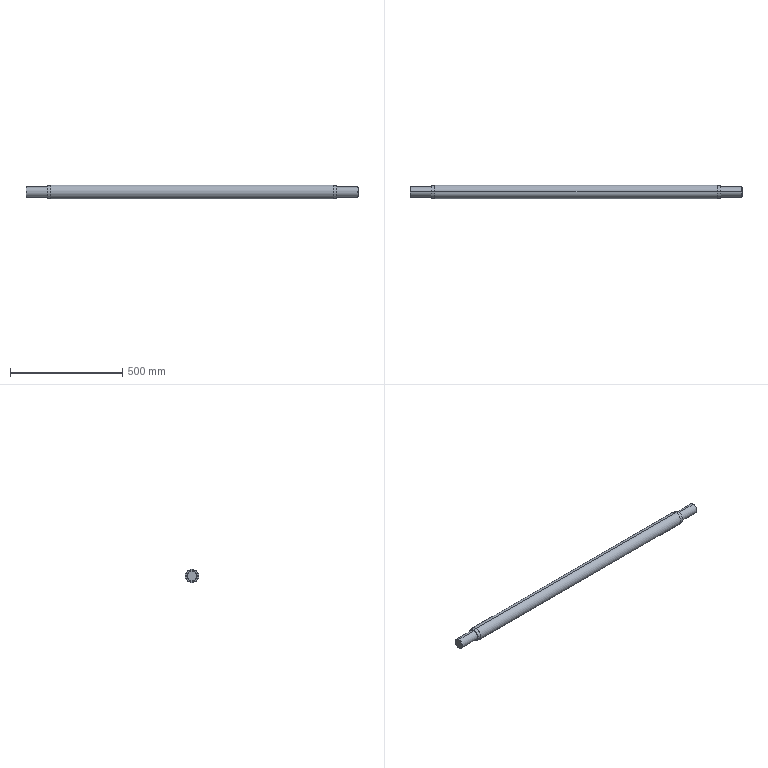Part | SolidWorks | features BaseBody 1 | 1 solid | 20 faces | box 1480 x 60 x 60 mm | volume 3935884 mm3 | cylinder 10 | plane 6 | cone 4 | commonest cylinder face diameters 45 x4 55 x4 60 x2
STEP:
#1=CARTESIAN_POINT('',(1595.073,277.036,21.5));
#2=VERTEX_POINT('',#1);
#3=CARTESIAN_POINT('',(1595.073,277.036,-21.5));
#4=VERTEX_POINT('',#3);
#5=CARTESIAN_POINT('',(1595.073,277.036,0.));
#6=DIRECTION('',(-1.,0.,0.));
#7=DIRECTION('',(0.,0.,1.));
#8=AXIS2_PLACEMENT_3D('',#5,#6,#7);
#9=CIRCLE('',#8,21.5);
#10=EDGE_CURVE('',#2,#4,#9,.T.);
#11=ORIENTED_EDGE('',*,*,#10,.T.);
#12=CARTESIAN_POINT('',(1594.073,277.036,-22.5));
#13=VERTEX_POINT('',#12);
#14=CARTESIAN_POINT('',(1595.073,277.036,-21.5));
#15=DIRECTION('',(-0.7071,0.,-0.7071));
#16=VECTOR('',#15,1000.);
#17=LINE('',#14,#16);
#18=EDGE_CURVE('',#4,#13,#17,.T.);
#19=ORIENTED_EDGE('',*,*,#18,.T.);
#20=CARTESIAN_POINT('',(1594.073,277.036,22.5));
#21=VERTEX_POINT('',#20);
#22=CARTESIAN_POINT('',(1594.073,277.036,0.));
#23=DIRECTION('',(-1.,0.,0.));
#24=DIRECTION('',(0.,0.,1.));
#25=AXIS2_PLACEMENT_3D('',#22,#23,#24);
#26=CIRCLE('',#25,22.5);
#27=EDGE_CURVE('',#21,#13,#26,.T.);
#28=ORIENTED_EDGE('',*,*,#27,.F.);
#29=CARTESIAN_POINT('',(1595.073,277.036,21.5));
#30=DIRECTION('',(-0.7071,0.,0.7071));
#31=VECTOR('',#30,1000.);
#32=LINE('',#29,#31);
#33=EDGE_CURVE('',#2,#21,#32,.T.);
#34=ORIENTED_EDGE('',*,*,#33,.F.);
#35=EDGE_LOOP('',(#11,#19,#28,#34));
#36=FACE_OUTER_BOUND('',#35,.T.);
#37=CARTESIAN_POINT('',(1595.073,277.036,0.));
#38=DIRECTION('',(-1.,0.,0.));
#39=DIRECTION('',(0.,0.,1.));
#40=AXIS2_PLACEMENT_3D('',#37,#38,#39);
#41=CONICAL_SURFACE('',#40,21.5,0.7854);
#42=ADVANCED_FACE('',(#36),#41,.T.);
#43=ORIENTED_EDGE('',*,*,#27,.T.);
#44=CARTESIAN_POINT('',(1500.073,277.036,-22.5));
#45=VERTEX_POINT('',#44);
#46=CARTESIAN_POINT('',(221.073,277.036,-22.5));
#47=DIRECTION('',(-1.,0.,0.));
#48=VECTOR('',#47,1000.);
#49=LINE('',#46,#48);
#50=EDGE_CURVE('',#13,#45,#49,.T.);
#51=ORIENTED_EDGE('',*,*,#50,.T.);
#52=CARTESIAN_POINT('',(1500.073,277.036,22.5));
#53=VERTEX_POINT('',#52);
#54=CARTESIAN_POINT('',(1500.073,277.036,0.));
#55=DIRECTION('',(-1.,0.,0.));
#56=DIRECTION('',(0.,0.,1.));
#57=AXIS2_PLACEMENT_3D('',#54,#55,#56);
#58=CIRCLE('',#57,22.5);
#59=EDGE_CURVE('',#53,#45,#58,.T.);
#60=ORIENTED_EDGE('',*,*,#59,.F.);
#61=CARTESIAN_POINT('',(221.073,277.036,22.5));
#62=DIRECTION('',(-1.,0.,0.));
#63=VECTOR('',#62,1000.);
#64=LINE('',#61,#63);
#65=EDGE_CURVE('',#21,#53,#64,.T.);
#66=ORIENTED_EDGE('',*,*,#65,.F.);
#67=EDGE_LOOP('',(#43,#51,#60,#66));
#68=FACE_OUTER_BOUND('',#67,.T.);
#69=CARTESIAN_POINT('',(221.073,277.036,0.));
#70=DIRECTION('',(-1.,0.,0.));
#71=DIRECTION('',(0.,0.,1.));
#72=AXIS2_PLACEMENT_3D('',#69,#70,#71);
#73=CYLINDRICAL_SURFACE('',#72,22.5);
#74=ADVANCED_FACE('',(#68),#73,.T.);
#75=CARTESIAN_POINT('',(1500.073,277.036,27.5));
#76=VERTEX_POINT('',#75);
#77=CARTESIAN_POINT('',(1500.073,277.036,-27.5));
#78=VERTEX_POINT('',#77);
#79=CARTESIAN_POINT('',(1500.073,277.036,0.));
#80=DIRECTION('',(-1.,0.,0.));
#81=DIRECTION('',(0.,0.,1.));
#82=AXIS2_PLACEMENT_3D('',#79,#80,#81);
#83=CIRCLE('',#82,27.5);
#84=EDGE_CURVE('',#76,#78,#83,.T.);
#85=ORIENTED_EDGE('',*,*,#84,.T.);
#86=CARTESIAN_POINT('',(1485.073,277.036,-27.5));
#87=VERTEX_POINT('',#86);
#88=CARTESIAN_POINT('',(221.073,277.036,-27.5));
#89=DIRECTION('',(-1.,0.,0.));
#90=VECTOR('',#89,1000.);
#91=LINE('',#88,#90);
#92=EDGE_CURVE('',#78,#87,#91,.T.);
#93=ORIENTED_EDGE('',*,*,#92,.T.);
#94=CARTESIAN_POINT('',(1485.073,277.036,27.5));
#95=VERTEX_POINT('',#94);
#96=CARTESIAN_POINT('',(1485.073,277.036,0.));
#97=DIRECTION('',(-1.,0.,0.));
#98=DIRECTION('',(0.,0.,1.));
#99=AXIS2_PLACEMENT_3D('',#96,#97,#98);
#100=CIRCLE('',#99,27.5);
#101=EDGE_CURVE('',#95,#87,#100,.T.);
#102=ORIENTED_EDGE('',*,*,#101,.F.);
#103=CARTESIAN_POINT('',(221.073,277.036,27.5));
#104=DIRECTION('',(-1.,0.,0.));
#105=VECTOR('',#104,1000.);
#106=LINE('',#103,#105);
#107=EDGE_CURVE('',#76,#95,#106,.T.);
#108=ORIENTED_EDGE('',*,*,#107,.F.);
#109=EDGE_LOOP('',(#85,#93,#102,#108));
#110=FACE_OUTER_BOUND('',#109,.T.);
#111=CARTESIAN_POINT('',(221.073,277.036,0.));
#112=DIRECTION('',(-1.,0.,0.));
#113=DIRECTION('',(0.,0.,1.));
#114=AXIS2_PLACEMENT_3D('',#111,#112,#113);
#115=CYLINDRICAL_SURFACE('',#114,27.5);
#116=ADVANCED_FACE('',(#110),#115,.T.);
#117=CARTESIAN_POINT('',(1485.073,277.036,30.));
#118=VERTEX_POINT('',#117);
#119=CARTESIAN_POINT('',(1485.073,277.036,-30.));
#120=VERTEX_POINT('',#119);
#121=CARTESIAN_POINT('',(1485.073,277.036,0.));
#122=DIRECTION('',(-1.,0.,0.));
#123=DIRECTION('',(0.,0.,1.));
#124=AXIS2_PLACEMENT_3D('',#121,#122,#123);
#125=CIRCLE('',#124,30.);
#126=EDGE_CURVE('',#118,#120,#125,.T.);
#127=ORIENTED_EDGE('',*,*,#126,.T.);
#128=CARTESIAN_POINT('',(225.073,277.036,-30.));
#129=VERTEX_POINT('',#128);
#130=CARTESIAN_POINT('',(221.073,277.036,-30.));
#131=DIRECTION('',(-1.,0.,0.));
#132=VECTOR('',#131,1000.);
#133=LINE('',#130,#132);
#134=EDGE_CURVE('',#120,#129,#133,.T.);
#135=ORIENTED_EDGE('',*,*,#134,.T.);
#136=CARTESIAN_POINT('',(225.073,277.036,30.));
#137=VERTEX_POINT('',#136);
#138=CARTESIAN_POINT('',(225.073,277.036,0.));
#139=DIRECTION('',(-1.,0.,0.));
#140=DIRECTION('',(0.,0.,1.));
#141=AXIS2_PLACEMENT_3D('',#138,#139,#140);
#142=CIRCLE('',#141,30.);
#143=EDGE_CURVE('',#137,#129,#142,.T.);
#144=ORIENTED_EDGE('',*,*,#143,.F.);
#145=CARTESIAN_POINT('',(221.073,277.036,30.));
#146=DIRECTION('',(-1.,0.,0.));
#147=VECTOR('',#146,1000.);
#148=LINE('',#145,#147);
#149=EDGE_CURVE('',#118,#137,#148,.T.);
#150=ORIENTED_EDGE('',*,*,#149,.F.);
#151=EDGE_LOOP('',(#127,#135,#144,#150));
#152=FACE_OUTER_BOUND('',#151,.T.);
#153=CARTESIAN_POINT('',(221.073,277.036,0.));
#154=DIRECTION('',(-1.,0.,0.));
#155=DIRECTION('',(0.,0.,1.));
#156=AXIS2_PLACEMENT_3D('',#153,#154,#155);
#157=CYLINDRICAL_SURFACE('',#156,30.);
#158=ADVANCED_FACE('',(#152),#157,.T.);
#159=CARTESIAN_POINT('',(225.073,277.036,27.5));
#160=VERTEX_POINT('',#159);
#161=CARTESIAN_POINT('',(225.073,277.036,-27.5));
#162=VERTEX_POINT('',#161);
#163=CARTESIAN_POINT('',(225.073,277.036,0.));
#164=DIRECTION('',(-1.,0.,0.));
#165=DIRECTION('',(0.,0.,1.));
#166=AXIS2_PLACEMENT_3D('',#163,#164,#165);
#167=CIRCLE('',#166,27.5);
#168=EDGE_CURVE('',#160,#162,#167,.T.);
#169=ORIENTED_EDGE('',*,*,#168,.T.);
#170=CARTESIAN_POINT('',(210.073,277.036,-27.5));
#171=VERTEX_POINT('',#170);
#172=CARTESIAN_POINT('',(221.073,277.036,-27.5));
#173=DIRECTION('',(-1.,0.,0.));
#174=VECTOR('',#173,1000.);
#175=LINE('',#172,#174);
#176=EDGE_CURVE('',#162,#171,#175,.T.);
#177=ORIENTED_EDGE('',*,*,#176,.T.);
#178=CARTESIAN_POINT('',(210.073,277.036,27.5));
#179=VERTEX_POINT('',#178);
#180=CARTESIAN_POINT('',(210.073,277.036,0.));
#181=DIRECTION('',(-1.,0.,0.));
#182=DIRECTION('',(0.,0.,1.));
#183=AXIS2_PLACEMENT_3D('',#180,#181,#182);
#184=CIRCLE('',#183,27.5);
#185=EDGE_CURVE('',#179,#171,#184,.T.);
#186=ORIENTED_EDGE('',*,*,#185,.F.);
#187=CARTESIAN_POINT('',(221.073,277.036,27.5));
#188=DIRECTION('',(-1.,0.,0.));
#189=VECTOR('',#188,1000.);
#190=LINE('',#187,#189);
#191=EDGE_CURVE('',#160,#179,#190,.T.);
#192=ORIENTED_EDGE('',*,*,#191,.F.);
#193=EDGE_LOOP('',(#169,#177,#186,#192));
#194=FACE_OUTER_BOUND('',#193,.T.);
#195=CARTESIAN_POINT('',(221.073,277.036,0.));
#196=DIRECTION('',(-1.,0.,0.));
#197=DIRECTION('',(0.,0.,1.));
#198=AXIS2_PLACEMENT_3D('',#195,#196,#197);
#199=CYLINDRICAL_SURFACE('',#198,27.5);
#200=ADVANCED_FACE('',(#194),#199,.T.);
#201=CARTESIAN_POINT('',(210.073,277.036,22.5));
#202=VERTEX_POINT('',#201);
#203=CARTESIAN_POINT('',(210.073,277.036,-22.5));
#204=VERTEX_POINT('',#203);
#205=CARTESIAN_POINT('',(210.073,277.036,0.));
#206=DIRECTION('',(-1.,0.,0.));
#207=DIRECTION('',(0.,0.,1.));
#208=AXIS2_PLACEMENT_3D('',#205,#206,#207);
#209=CIRCLE('',#208,22.5);
#210=EDGE_CURVE('',#202,#204,#209,.T.);
#211=ORIENTED_EDGE('',*,*,#210,.T.);
#212=CARTESIAN_POINT('',(116.073,277.036,-22.5));
#213=VERTEX_POINT('',#212);
#214=CARTESIAN_POINT('',(221.073,277.036,-22.5));
#215=DIRECTION('',(-1.,0.,0.));
#216=VECTOR('',#215,1000.);
#217=LINE('',#214,#216);
#218=EDGE_CURVE('',#204,#213,#217,.T.);
#219=ORIENTED_EDGE('',*,*,#218,.T.);
#220=CARTESIAN_POINT('',(116.073,277.036,22.5));
#221=VERTEX_POINT('',#220);
#222=CARTESIAN_POINT('',(116.073,277.036,0.));
#223=DIRECTION('',(-1.,0.,0.));
#224=DIRECTION('',(0.,0.,1.));
#225=AXIS2_PLACEMENT_3D('',#222,#223,#224);
#226=CIRCLE('',#225,22.5);
#227=EDGE_CURVE('',#221,#213,#226,.T.);
#228=ORIENTED_EDGE('',*,*,#227,.F.);
#229=CARTESIAN_POINT('',(221.073,277.036,22.5));
#230=DIRECTION('',(-1.,0.,0.));
#231=VECTOR('',#230,1000.);
#232=LINE('',#229,#231);
#233=EDGE_CURVE('',#202,#221,#232,.T.);
#234=ORIENTED_EDGE('',*,*,#233,.F.);
#235=EDGE_LOOP('',(#211,#219,#228,#234));
#236=FACE_OUTER_BOUND('',#235,.T.);
#237=CARTESIAN_POINT('',(221.073,277.036,0.));
#238=DIRECTION('',(-1.,0.,0.));
#239=DIRECTION('',(0.,0.,1.));
#240=AXIS2_PLACEMENT_3D('',#237,#238,#239);
#241=CYLINDRICAL_SURFACE('',#240,22.5);
#242=ADVANCED_FACE('',(#236),#241,.T.);
#243=CARTESIAN_POINT('',(115.073,277.036,21.5));
#244=VERTEX_POINT('',#243);
#245=CARTESIAN_POINT('',(115.073,277.036,-21.5));
#246=VERTEX_POINT('',#245);
#247=CARTESIAN_POINT('',(115.073,277.036,0.));
#248=DIRECTION('',(-1.,0.,0.));
#249=DIRECTION('',(0.,0.,1.));
#250=AXIS2_PLACEMENT_3D('',#247,#248,#249);
#251=CIRCLE('',#250,21.5);
#252=EDGE_CURVE('',#244,#246,#251,.T.);
#253=ORIENTED_EDGE('',*,*,#252,.F.);
#254=CARTESIAN_POINT('',(116.073,277.036,22.5));
#255=DIRECTION('',(0.7071,0.,0.7071));
#256=VECTOR('',#255,1000.);
#257=LINE('',#254,#256);
#258=EDGE_CURVE('',#244,#221,#257,.T.);
#259=ORIENTED_EDGE('',*,*,#258,.T.);
#260=ORIENTED_EDGE('',*,*,#227,.T.);
#261=CARTESIAN_POINT('',(116.073,277.036,-22.5));
#262=DIRECTION('',(0.7071,0.,-0.7071));
#263=VECTOR('',#262,1000.);
#264=LINE('',#261,#263);
#265=EDGE_CURVE('',#246,#213,#264,.T.);
#266=ORIENTED_EDGE('',*,*,#265,.F.);
#267=EDGE_LOOP('',(#253,#259,#260,#266));
#268=FACE_OUTER_BOUND('',#267,.T.);
#269=CARTESIAN_POINT('',(116.073,277.036,0.));
#270=DIRECTION('',(1.,0.,0.));
#271=DIRECTION('',(0.,0.,-1.));
#272=AXIS2_PLACEMENT_3D('',#269,#270,#271);
#273=CONICAL_SURFACE('',#272,22.5,0.7854);
#274=ADVANCED_FACE('',(#268),#273,.T.);
#275=CARTESIAN_POINT('',(115.073,277.036,0.));
#276=DIRECTION('',(-1.,0.,0.));
#277=DIRECTION('',(0.,0.,1.));
#278=AXIS2_PLACEMENT_3D('',#275,#276,#277);
#279=CIRCLE('',#278,21.5);
#280=EDGE_CURVE('',#246,#244,#279,.T.);
#281=ORIENTED_EDGE('',*,*,#280,.T.);
#282=ORIENTED_EDGE('',*,*,#252,.T.);
#283=EDGE_LOOP('',(#281,#282));
#284=FACE_OUTER_BOUND('',#283,.T.);
#285=CARTESIAN_POINT('',(115.073,277.036,0.));
#286=DIRECTION('',(1.,0.,0.));
#287=DIRECTION('',(0.,0.,-1.));
#288=AXIS2_PLACEMENT_3D('',#285,#286,#287);
#289=PLANE('',#288);
#290=ADVANCED_FACE('',(#284),#289,.F.);
#291=ORIENTED_EDGE('',*,*,#258,.F.);
#292=ORIENTED_EDGE('',*,*,#280,.F.);
#293=ORIENTED_EDGE('',*,*,#265,.T.);
#294=CARTESIAN_POINT('',(116.073,277.036,0.));
#295=DIRECTION('',(-1.,0.,0.));
#296=DIRECTION('',(0.,0.,1.));
#297=AXIS2_PLACEMENT_3D('',#294,#295,#296);
#298=CIRCLE('',#297,22.5);
#299=EDGE_CURVE('',#213,#221,#298,.T.);
#300=ORIENTED_EDGE('',*,*,#299,.T.);
#301=EDGE_LOOP('',(#291,#292,#293,#300));
#302=FACE_OUTER_BOUND('',#301,.T.);
#303=CARTESIAN_POINT('',(116.073,277.036,0.));
#304=DIRECTION('',(1.,0.,0.));
#305=DIRECTION('',(0.,0.,-1.));
#306=AXIS2_PLACEMENT_3D('',#303,#304,#305);
#307=CONICAL_SURFACE('',#306,22.5,0.7854);
#308=ADVANCED_FACE('',(#302),#307,.T.);
#309=ORIENTED_EDGE('',*,*,#218,.F.);
#310=CARTESIAN_POINT('',(210.073,277.036,0.));
#311=DIRECTION('',(-1.,0.,0.));
#312=DIRECTION('',(0.,0.,1.));
#313=AXIS2_PLACEMENT_3D('',#310,#311,#312);
#314=CIRCLE('',#313,22.5);
#315=EDGE_CURVE('',#204,#202,#314,.T.);
#316=ORIENTED_EDGE('',*,*,#315,.T.);
#317=ORIENTED_EDGE('',*,*,#233,.T.);
#318=ORIENTED_EDGE('',*,*,#299,.F.);
#319=EDGE_LOOP('',(#309,#316,#317,#318));
#320=FACE_OUTER_BOUND('',#319,.T.);
#321=CARTESIAN_POINT('',(221.073,277.036,0.));
#322=DIRECTION('',(-1.,0.,0.));
#323=DIRECTION('',(0.,0.,1.));
#324=AXIS2_PLACEMENT_3D('',#321,#322,#323);
#325=CYLINDRICAL_SURFACE('',#324,22.5);
#326=ADVANCED_FACE('',(#320),#325,.T.);
#327=ORIENTED_EDGE('',*,*,#210,.F.);
#328=ORIENTED_EDGE('',*,*,#315,.F.);
#329=EDGE_LOOP('',(#327,#328));
#330=FACE_BOUND('',#329,.T.);
#331=ORIENTED_EDGE('',*,*,#185,.T.);
#332=CARTESIAN_POINT('',(210.073,277.036,0.));
#333=DIRECTION('',(-1.,0.,0.));
#334=DIRECTION('',(0.,0.,1.));
#335=AXIS2_PLACEMENT_3D('',#332,#333,#334);
#336=CIRCLE('',#335,27.5);
#337=EDGE_CURVE('',#171,#179,#336,.T.);
#338=ORIENTED_EDGE('',*,*,#337,.T.);
#339=EDGE_LOOP('',(#331,#338));
#340=FACE_OUTER_BOUND('',#339,.T.);
#341=CARTESIAN_POINT('',(210.073,299.536,0.));
#342=DIRECTION('',(1.,0.,0.));
#343=DIRECTION('',(0.,0.,-1.));
#344=AXIS2_PLACEMENT_3D('',#341,#342,#343);
#345=PLANE('',#344);
#346=ADVANCED_FACE('',(#330,#340),#345,.F.);
#347=ORIENTED_EDGE('',*,*,#176,.F.);
#348=CARTESIAN_POINT('',(225.073,277.036,0.));
#349=DIRECTION('',(-1.,0.,0.));
#350=DIRECTION('',(0.,0.,1.));
#351=AXIS2_PLACEMENT_3D('',#348,#349,#350);
#352=CIRCLE('',#351,27.5);
#353=EDGE_CURVE('',#162,#160,#352,.T.);
#354=ORIENTED_EDGE('',*,*,#353,.T.);
#355=ORIENTED_EDGE('',*,*,#191,.T.);
#356=ORIENTED_EDGE('',*,*,#337,.F.);
#357=EDGE_LOOP('',(#347,#354,#355,#356));
#358=FACE_OUTER_BOUND('',#357,.T.);
#359=CARTESIAN_POINT('',(221.073,277.036,0.));
#360=DIRECTION('',(-1.,0.,0.));
#361=DIRECTION('',(0.,0.,1.));
#362=AXIS2_PLACEMENT_3D('',#359,#360,#361);
#363=CYLINDRICAL_SURFACE('',#362,27.5);
#364=ADVANCED_FACE('',(#358),#363,.T.);
#365=ORIENTED_EDGE('',*,*,#168,.F.);
#366=ORIENTED_EDGE('',*,*,#353,.F.);
#367=EDGE_LOOP('',(#365,#366));
#368=FACE_BOUND('',#367,.T.);
#369=ORIENTED_EDGE('',*,*,#143,.T.);
#370=CARTESIAN_POINT('',(225.073,277.036,0.));
#371=DIRECTION('',(-1.,0.,0.));
#372=DIRECTION('',(0.,0.,1.));
#373=AXIS2_PLACEMENT_3D('',#370,#371,#372);
#374=CIRCLE('',#373,30.);
#375=EDGE_CURVE('',#129,#137,#374,.T.);
#376=ORIENTED_EDGE('',*,*,#375,.T.);
#377=EDGE_LOOP('',(#369,#376));
#378=FACE_OUTER_BOUND('',#377,.T.);
#379=CARTESIAN_POINT('',(225.073,304.536,0.));
#380=DIRECTION('',(1.,0.,0.));
#381=DIRECTION('',(0.,0.,-1.));
#382=AXIS2_PLACEMENT_3D('',#379,#380,#381);
#383=PLANE('',#382);
#384=ADVANCED_FACE('',(#368,#378),#383,.F.);
#385=ORIENTED_EDGE('',*,*,#134,.F.);
#386=CARTESIAN_POINT('',(1485.073,277.036,0.));
#387=DIRECTION('',(-1.,0.,0.));
#388=DIRECTION('',(0.,0.,1.));
#389=AXIS2_PLACEMENT_3D('',#386,#387,#388);
#390=CIRCLE('',#389,30.);
#391=EDGE_CURVE('',#120,#118,#390,.T.);
#392=ORIENTED_EDGE('',*,*,#391,.T.);
#393=ORIENTED_EDGE('',*,*,#149,.T.);
#394=ORIENTED_EDGE('',*,*,#375,.F.);
#395=EDGE_LOOP('',(#385,#392,#393,#394));
#396=FACE_OUTER_BOUND('',#395,.T.);
#397=CARTESIAN_POINT('',(221.073,277.036,0.));
#398=DIRECTION('',(-1.,0.,0.));
#399=DIRECTION('',(0.,0.,1.));
#400=AXIS2_PLACEMENT_3D('',#397,#398,#399);
#401=CYLINDRICAL_SURFACE('',#400,30.);
#402=ADVANCED_FACE('',(#396),#401,.T.);
#403=ORIENTED_EDGE('',*,*,#126,.F.);
#404=ORIENTED_EDGE('',*,*,#391,.F.);
#405=EDGE_LOOP('',(#403,#404));
#406=FACE_OUTER_BOUND('',#405,.T.);
#407=ORIENTED_EDGE('',*,*,#101,.T.);
#408=CARTESIAN_POINT('',(1485.073,277.036,0.));
#409=DIRECTION('',(-1.,0.,0.));
#410=DIRECTION('',(0.,0.,1.));
#411=AXIS2_PLACEMENT_3D('',#408,#409,#410);
#412=CIRCLE('',#411,27.5);
#413=EDGE_CURVE('',#87,#95,#412,.T.);
#414=ORIENTED_EDGE('',*,*,#413,.T.);
#415=EDGE_LOOP('',(#407,#414));
#416=FACE_BOUND('',#415,.T.);
#417=CARTESIAN_POINT('',(1485.073,307.036,0.));
#418=DIRECTION('',(-1.,0.,0.));
#419=DIRECTION('',(0.,0.,1.));
#420=AXIS2_PLACEMENT_3D('',#417,#418,#419);
#421=PLANE('',#420);
#422=ADVANCED_FACE('',(#406,#416),#421,.F.);
#423=ORIENTED_EDGE('',*,*,#92,.F.);
#424=CARTESIAN_POINT('',(1500.073,277.036,0.));
#425=DIRECTION('',(-1.,0.,0.));
#426=DIRECTION('',(0.,0.,1.));
#427=AXIS2_PLACEMENT_3D('',#424,#425,#426);
#428=CIRCLE('',#427,27.5);
#429=EDGE_CURVE('',#78,#76,#428,.T.);
#430=ORIENTED_EDGE('',*,*,#429,.T.);
#431=ORIENTED_EDGE('',*,*,#107,.T.);
#432=ORIENTED_EDGE('',*,*,#413,.F.);
#433=EDGE_LOOP('',(#423,#430,#431,#432));
#434=FACE_OUTER_BOUND('',#433,.T.);
#435=CARTESIAN_POINT('',(221.073,277.036,0.));
#436=DIRECTION('',(-1.,0.,0.));
#437=DIRECTION('',(0.,0.,1.));
#438=AXIS2_PLACEMENT_3D('',#435,#436,#437);
#439=CYLINDRICAL_SURFACE('',#438,27.5);
#440=ADVANCED_FACE('',(#434),#439,.T.);
#441=ORIENTED_EDGE('',*,*,#84,.F.);
#442=ORIENTED_EDGE('',*,*,#429,.F.);
#443=EDGE_LOOP('',(#441,#442));
#444=FACE_OUTER_BOUND('',#443,.T.);
#445=ORIENTED_EDGE('',*,*,#59,.T.);
#446=CARTESIAN_POINT('',(1500.073,277.036,0.));
#447=DIRECTION('',(-1.,0.,0.));
#448=DIRECTION('',(0.,0.,1.));
#449=AXIS2_PLACEMENT_3D('',#446,#447,#448);
#450=CIRCLE('',#449,22.5);
#451=EDGE_CURVE('',#45,#53,#450,.T.);
#452=ORIENTED_EDGE('',*,*,#451,.T.);
#453=EDGE_LOOP('',(#445,#452));
#454=FACE_BOUND('',#453,.T.);
#455=CARTESIAN_POINT('',(1500.073,304.536,0.));
#456=DIRECTION('',(-1.,0.,0.));
#457=DIRECTION('',(0.,0.,1.));
#458=AXIS2_PLACEMENT_3D('',#455,#456,#457);
#459=PLANE('',#458);
#460=ADVANCED_FACE('',(#444,#454),#459,.F.);
#461=ORIENTED_EDGE('',*,*,#50,.F.);
#462=CARTESIAN_POINT('',(1594.073,277.036,0.));
#463=DIRECTION('',(-1.,0.,0.));
#464=DIRECTION('',(0.,0.,1.));
#465=AXIS2_PLACEMENT_3D('',#462,#463,#464);
#466=CIRCLE('',#465,22.5);
#467=EDGE_CURVE('',#13,#21,#466,.T.);
#468=ORIENTED_EDGE('',*,*,#467,.T.);
#469=ORIENTED_EDGE('',*,*,#65,.T.);
#470=ORIENTED_EDGE('',*,*,#451,.F.);
#471=EDGE_LOOP('',(#461,#468,#469,#470));
#472=FACE_OUTER_BOUND('',#471,.T.);
#473=CARTESIAN_POINT('',(221.073,277.036,0.));
#474=DIRECTION('',(-1.,0.,0.));
#475=DIRECTION('',(0.,0.,1.));
#476=AXIS2_PLACEMENT_3D('',#473,#474,#475);
#477=CYLINDRICAL_SURFACE('',#476,22.5);
#478=ADVANCED_FACE('',(#472),#477,.T.);
#479=ORIENTED_EDGE('',*,*,#18,.F.);
#480=CARTESIAN_POINT('',(1595.073,277.036,0.));
#481=DIRECTION('',(-1.,0.,0.));
#482=DIRECTION('',(0.,0.,1.));
#483=AXIS2_PLACEMENT_3D('',#480,#481,#482);
#484=CIRCLE('',#483,21.5);
#485=EDGE_CURVE('',#4,#2,#484,.T.);
#486=ORIENTED_EDGE('',*,*,#485,.T.);
#487=ORIENTED_EDGE('',*,*,#33,.T.);
#488=ORIENTED_EDGE('',*,*,#467,.F.);
#489=EDGE_LOOP('',(#479,#486,#487,#488));
#490=FACE_OUTER_BOUND('',#489,.T.);
#491=CARTESIAN_POINT('',(1595.073,277.036,0.));
#492=DIRECTION('',(-1.,0.,0.));
#493=DIRECTION('',(0.,0.,1.));
#494=AXIS2_PLACEMENT_3D('',#491,#492,#493);
#495=CONICAL_SURFACE('',#494,21.5,0.7854);
#496=ADVANCED_FACE('',(#490),#495,.T.);
#497=ORIENTED_EDGE('',*,*,#10,.F.);
#498=ORIENTED_EDGE('',*,*,#485,.F.);
#499=EDGE_LOOP('',(#497,#498));
#500=FACE_OUTER_BOUND('',#499,.T.);
#501=CARTESIAN_POINT('',(1595.073,298.536,0.));
#502=DIRECTION('',(-1.,0.,0.));
#503=DIRECTION('',(0.,0.,1.));
#504=AXIS2_PLACEMENT_3D('',#501,#502,#503);
#505=PLANE('',#504);
#506=ADVANCED_FACE('',(#500),#505,.F.);
#507=CLOSED_SHELL('',(#42,#74,#116,#158,#200,#242,#274,#290,#308,#326,#346,#364,#384,#402,#422,#440,#460,#478,#496,#506));
#508=MANIFOLD_SOLID_BREP('',#507);
#509=CARTESIAN_POINT('',(0.,0.,0.));
#510=DIRECTION('',(0.,0.,1.));
#511=DIRECTION('',(1.,0.,0.));
#512=AXIS2_PLACEMENT_3D('',#509,#510,#511);
#513=(LENGTH_UNIT()NAMED_UNIT(*)SI_UNIT(.MILLI.,.METRE.));
#514=UNCERTAINTY_MEASURE_WITH_UNIT(LENGTH_MEASURE(0.00001),#513,'','');
#515=(NAMED_UNIT(*)PLANE_ANGLE_UNIT()SI_UNIT($,.RADIAN.));
#516=(NAMED_UNIT(*)SI_UNIT($,.STERADIAN.)SOLID_ANGLE_UNIT());
#517=(GEOMETRIC_REPRESENTATION_CONTEXT(3)GLOBAL_UNCERTAINTY_ASSIGNED_CONTEXT((#514))GLOBAL_UNIT_ASSIGNED_CONTEXT((#513,#515,#516))REPRESENTATION_CONTEXT('',''));
#518=ADVANCED_BREP_SHAPE_REPRESENTATION('',(#508,#512),#517);